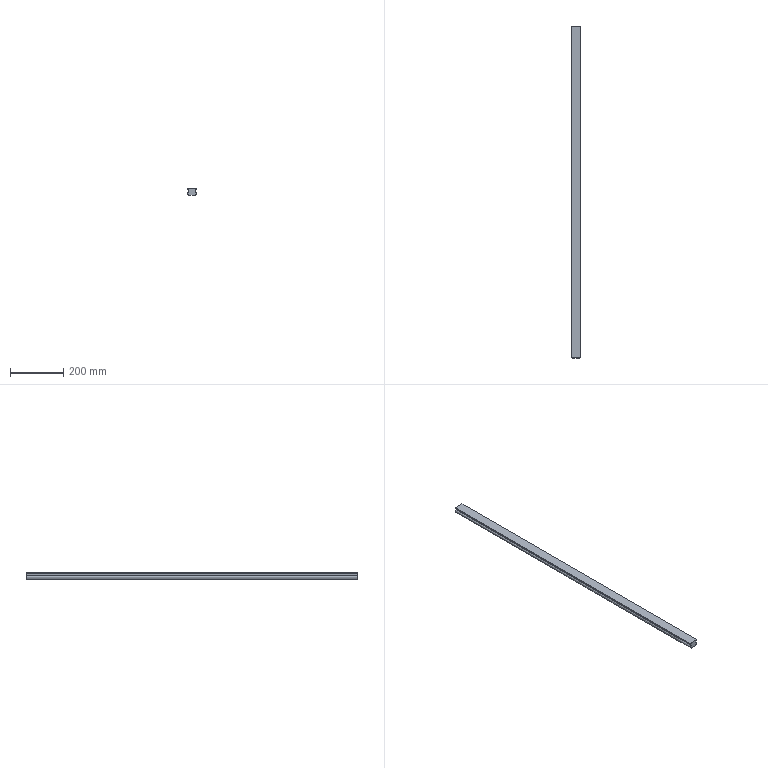Part | SolidWorks | features Extrusion 1 | 1 solid | 14 faces | box 36 x 1252 x 25 mm | volume 935920 mm3 | plane 12 | cylinder 2 | commonest cylinder face diameters 10 x2
STEP:
#1=CARTESIAN_POINT('',(12.5,0.,5.));
#2=VERTEX_POINT('',#1);
#3=CARTESIAN_POINT('',(12.5,0.,-5.));
#4=VERTEX_POINT('',#3);
#5=CARTESIAN_POINT('',(12.5,0.,0.));
#6=DIRECTION('',(0.,1.,0.));
#7=DIRECTION('',(0.,0.,1.));
#8=AXIS2_PLACEMENT_3D('',#5,#6,#7);
#9=CIRCLE('',#8,5.);
#10=EDGE_CURVE('',#2,#4,#9,.T.);
#11=ORIENTED_EDGE('',*,*,#10,.T.);
#12=CARTESIAN_POINT('',(12.5,1252.,-5.));
#13=VERTEX_POINT('',#12);
#14=CARTESIAN_POINT('',(12.5,1252.,-5.));
#15=DIRECTION('',(0.,-1.,0.));
#16=VECTOR('',#15,1000.);
#17=LINE('',#14,#16);
#18=EDGE_CURVE('',#13,#4,#17,.T.);
#19=ORIENTED_EDGE('',*,*,#18,.F.);
#20=CARTESIAN_POINT('',(12.5,1252.,5.));
#21=VERTEX_POINT('',#20);
#22=CARTESIAN_POINT('',(12.5,1252.,0.));
#23=DIRECTION('',(0.,1.,0.));
#24=DIRECTION('',(0.,0.,1.));
#25=AXIS2_PLACEMENT_3D('',#22,#23,#24);
#26=CIRCLE('',#25,5.);
#27=EDGE_CURVE('',#21,#13,#26,.T.);
#28=ORIENTED_EDGE('',*,*,#27,.F.);
#29=CARTESIAN_POINT('',(12.5,1252.,5.));
#30=DIRECTION('',(0.,-1.,0.));
#31=VECTOR('',#30,1000.);
#32=LINE('',#29,#31);
#33=EDGE_CURVE('',#21,#2,#32,.T.);
#34=ORIENTED_EDGE('',*,*,#33,.T.);
#35=EDGE_LOOP('',(#11,#19,#28,#34));
#36=FACE_OUTER_BOUND('',#35,.T.);
#37=CARTESIAN_POINT('',(12.5,1252.,0.));
#38=DIRECTION('',(0.,-1.,0.));
#39=DIRECTION('',(0.,0.,-1.));
#40=AXIS2_PLACEMENT_3D('',#37,#38,#39);
#41=CYLINDRICAL_SURFACE('',#40,5.);
#42=ADVANCED_FACE('',(#36),#41,.T.);
#43=CARTESIAN_POINT('',(12.5,0.,-8.));
#44=VERTEX_POINT('',#43);
#45=CARTESIAN_POINT('',(12.5,0.,-8.));
#46=DIRECTION('',(0.,0.,-1.));
#47=VECTOR('',#46,1000.);
#48=LINE('',#45,#47);
#49=EDGE_CURVE('',#4,#44,#48,.T.);
#50=ORIENTED_EDGE('',*,*,#49,.T.);
#51=CARTESIAN_POINT('',(12.5,1252.,-8.));
#52=VERTEX_POINT('',#51);
#53=CARTESIAN_POINT('',(12.5,1252.,-8.));
#54=DIRECTION('',(0.,-1.,0.));
#55=VECTOR('',#54,1000.);
#56=LINE('',#53,#55);
#57=EDGE_CURVE('',#52,#44,#56,.T.);
#58=ORIENTED_EDGE('',*,*,#57,.F.);
#59=CARTESIAN_POINT('',(12.5,1252.,-8.));
#60=DIRECTION('',(0.,0.,-1.));
#61=VECTOR('',#60,1000.);
#62=LINE('',#59,#61);
#63=EDGE_CURVE('',#13,#52,#62,.T.);
#64=ORIENTED_EDGE('',*,*,#63,.F.);
#65=ORIENTED_EDGE('',*,*,#18,.T.);
#66=EDGE_LOOP('',(#50,#58,#64,#65));
#67=FACE_OUTER_BOUND('',#66,.T.);
#68=CARTESIAN_POINT('',(12.5,1252.,-8.));
#69=DIRECTION('',(-1.,0.,0.));
#70=DIRECTION('',(0.,0.,1.));
#71=AXIS2_PLACEMENT_3D('',#68,#69,#70);
#72=PLANE('',#71);
#73=ADVANCED_FACE('',(#67),#72,.F.);
#74=CARTESIAN_POINT('',(-12.5,0.,-8.));
#75=VERTEX_POINT('',#74);
#76=CARTESIAN_POINT('',(-12.5,0.,-8.));
#77=DIRECTION('',(-1.,0.,0.));
#78=VECTOR('',#77,1000.);
#79=LINE('',#76,#78);
#80=EDGE_CURVE('',#44,#75,#79,.T.);
#81=ORIENTED_EDGE('',*,*,#80,.T.);
#82=CARTESIAN_POINT('',(-12.5,1252.,-8.));
#83=VERTEX_POINT('',#82);
#84=CARTESIAN_POINT('',(-12.5,1252.,-8.));
#85=DIRECTION('',(0.,-1.,0.));
#86=VECTOR('',#85,1000.);
#87=LINE('',#84,#86);
#88=EDGE_CURVE('',#83,#75,#87,.T.);
#89=ORIENTED_EDGE('',*,*,#88,.F.);
#90=CARTESIAN_POINT('',(-12.5,1252.,-8.));
#91=DIRECTION('',(-1.,0.,0.));
#92=VECTOR('',#91,1000.);
#93=LINE('',#90,#92);
#94=EDGE_CURVE('',#52,#83,#93,.T.);
#95=ORIENTED_EDGE('',*,*,#94,.F.);
#96=ORIENTED_EDGE('',*,*,#57,.T.);
#97=EDGE_LOOP('',(#81,#89,#95,#96));
#98=FACE_OUTER_BOUND('',#97,.T.);
#99=CARTESIAN_POINT('',(-12.5,1252.,-8.));
#100=DIRECTION('',(0.,0.,1.));
#101=DIRECTION('',(1.,0.,0.));
#102=AXIS2_PLACEMENT_3D('',#99,#100,#101);
#103=PLANE('',#102);
#104=ADVANCED_FACE('',(#98),#103,.F.);
#105=CARTESIAN_POINT('',(-12.5,0.,-5.));
#106=VERTEX_POINT('',#105);
#107=CARTESIAN_POINT('',(-12.5,0.,-5.));
#108=DIRECTION('',(0.,0.,1.));
#109=VECTOR('',#108,1000.);
#110=LINE('',#107,#109);
#111=EDGE_CURVE('',#75,#106,#110,.T.);
#112=ORIENTED_EDGE('',*,*,#111,.T.);
#113=CARTESIAN_POINT('',(-12.5,1252.,-5.));
#114=VERTEX_POINT('',#113);
#115=CARTESIAN_POINT('',(-12.5,1252.,-5.));
#116=DIRECTION('',(0.,-1.,0.));
#117=VECTOR('',#116,1000.);
#118=LINE('',#115,#117);
#119=EDGE_CURVE('',#114,#106,#118,.T.);
#120=ORIENTED_EDGE('',*,*,#119,.F.);
#121=CARTESIAN_POINT('',(-12.5,1252.,-5.));
#122=DIRECTION('',(0.,0.,1.));
#123=VECTOR('',#122,1000.);
#124=LINE('',#121,#123);
#125=EDGE_CURVE('',#83,#114,#124,.T.);
#126=ORIENTED_EDGE('',*,*,#125,.F.);
#127=ORIENTED_EDGE('',*,*,#88,.T.);
#128=EDGE_LOOP('',(#112,#120,#126,#127));
#129=FACE_OUTER_BOUND('',#128,.T.);
#130=CARTESIAN_POINT('',(-12.5,1252.,-5.));
#131=DIRECTION('',(1.,0.,0.));
#132=DIRECTION('',(0.,0.,-1.));
#133=AXIS2_PLACEMENT_3D('',#130,#131,#132);
#134=PLANE('',#133);
#135=ADVANCED_FACE('',(#129),#134,.F.);
#136=CARTESIAN_POINT('',(-12.5,0.,5.));
#137=VERTEX_POINT('',#136);
#138=CARTESIAN_POINT('',(-12.5,0.,0.));
#139=DIRECTION('',(0.,1.,0.));
#140=DIRECTION('',(0.,0.,1.));
#141=AXIS2_PLACEMENT_3D('',#138,#139,#140);
#142=CIRCLE('',#141,5.);
#143=EDGE_CURVE('',#106,#137,#142,.T.);
#144=ORIENTED_EDGE('',*,*,#143,.T.);
#145=CARTESIAN_POINT('',(-12.5,1252.,5.));
#146=VERTEX_POINT('',#145);
#147=CARTESIAN_POINT('',(-12.5,1252.,5.));
#148=DIRECTION('',(0.,-1.,0.));
#149=VECTOR('',#148,1000.);
#150=LINE('',#147,#149);
#151=EDGE_CURVE('',#146,#137,#150,.T.);
#152=ORIENTED_EDGE('',*,*,#151,.F.);
#153=CARTESIAN_POINT('',(-12.5,1252.,0.));
#154=DIRECTION('',(0.,1.,0.));
#155=DIRECTION('',(0.,0.,1.));
#156=AXIS2_PLACEMENT_3D('',#153,#154,#155);
#157=CIRCLE('',#156,5.);
#158=EDGE_CURVE('',#114,#146,#157,.T.);
#159=ORIENTED_EDGE('',*,*,#158,.F.);
#160=ORIENTED_EDGE('',*,*,#119,.T.);
#161=EDGE_LOOP('',(#144,#152,#159,#160));
#162=FACE_OUTER_BOUND('',#161,.T.);
#163=CARTESIAN_POINT('',(-12.5,1252.,0.));
#164=DIRECTION('',(0.,-1.,0.));
#165=DIRECTION('',(0.,0.,-1.));
#166=AXIS2_PLACEMENT_3D('',#163,#164,#165);
#167=CYLINDRICAL_SURFACE('',#166,5.);
#168=ADVANCED_FACE('',(#162),#167,.T.);
#169=CARTESIAN_POINT('',(-12.5,0.,13.));
#170=VERTEX_POINT('',#169);
#171=CARTESIAN_POINT('',(-12.5,0.,5.));
#172=DIRECTION('',(0.,0.,1.));
#173=VECTOR('',#172,1000.);
#174=LINE('',#171,#173);
#175=EDGE_CURVE('',#137,#170,#174,.T.);
#176=ORIENTED_EDGE('',*,*,#175,.T.);
#177=CARTESIAN_POINT('',(-12.5,1252.,13.));
#178=VERTEX_POINT('',#177);
#179=CARTESIAN_POINT('',(-12.5,1252.,13.));
#180=DIRECTION('',(0.,-1.,0.));
#181=VECTOR('',#180,1000.);
#182=LINE('',#179,#181);
#183=EDGE_CURVE('',#178,#170,#182,.T.);
#184=ORIENTED_EDGE('',*,*,#183,.F.);
#185=CARTESIAN_POINT('',(-12.5,1252.,5.));
#186=DIRECTION('',(0.,0.,1.));
#187=VECTOR('',#186,1000.);
#188=LINE('',#185,#187);
#189=EDGE_CURVE('',#146,#178,#188,.T.);
#190=ORIENTED_EDGE('',*,*,#189,.F.);
#191=ORIENTED_EDGE('',*,*,#151,.T.);
#192=EDGE_LOOP('',(#176,#184,#190,#191));
#193=FACE_OUTER_BOUND('',#192,.T.);
#194=CARTESIAN_POINT('',(-12.5,1252.,5.));
#195=DIRECTION('',(1.,0.,0.));
#196=DIRECTION('',(0.,0.,-1.));
#197=AXIS2_PLACEMENT_3D('',#194,#195,#196);
#198=PLANE('',#197);
#199=ADVANCED_FACE('',(#193),#198,.F.);
#200=CARTESIAN_POINT('',(-18.,0.,13.));
#201=VERTEX_POINT('',#200);
#202=CARTESIAN_POINT('',(-12.5,0.,13.));
#203=DIRECTION('',(-1.,0.,0.));
#204=VECTOR('',#203,1000.);
#205=LINE('',#202,#204);
#206=EDGE_CURVE('',#170,#201,#205,.T.);
#207=ORIENTED_EDGE('',*,*,#206,.T.);
#208=CARTESIAN_POINT('',(-18.,1252.,13.));
#209=VERTEX_POINT('',#208);
#210=CARTESIAN_POINT('',(-18.,1252.,13.));
#211=DIRECTION('',(0.,-1.,0.));
#212=VECTOR('',#211,1000.);
#213=LINE('',#210,#212);
#214=EDGE_CURVE('',#209,#201,#213,.T.);
#215=ORIENTED_EDGE('',*,*,#214,.F.);
#216=CARTESIAN_POINT('',(-12.5,1252.,13.));
#217=DIRECTION('',(-1.,0.,0.));
#218=VECTOR('',#217,1000.);
#219=LINE('',#216,#218);
#220=EDGE_CURVE('',#178,#209,#219,.T.);
#221=ORIENTED_EDGE('',*,*,#220,.F.);
#222=ORIENTED_EDGE('',*,*,#183,.T.);
#223=EDGE_LOOP('',(#207,#215,#221,#222));
#224=FACE_OUTER_BOUND('',#223,.T.);
#225=CARTESIAN_POINT('',(-12.5,1252.,13.));
#226=DIRECTION('',(0.,0.,1.));
#227=DIRECTION('',(1.,0.,0.));
#228=AXIS2_PLACEMENT_3D('',#225,#226,#227);
#229=PLANE('',#228);
#230=ADVANCED_FACE('',(#224),#229,.F.);
#231=CARTESIAN_POINT('',(-18.,0.,17.));
#232=VERTEX_POINT('',#231);
#233=CARTESIAN_POINT('',(-18.,0.,13.));
#234=DIRECTION('',(0.,0.,1.));
#235=VECTOR('',#234,1000.);
#236=LINE('',#233,#235);
#237=EDGE_CURVE('',#201,#232,#236,.T.);
#238=ORIENTED_EDGE('',*,*,#237,.T.);
#239=CARTESIAN_POINT('',(-18.,1252.,17.));
#240=VERTEX_POINT('',#239);
#241=CARTESIAN_POINT('',(-18.,1252.,17.));
#242=DIRECTION('',(0.,-1.,0.));
#243=VECTOR('',#242,1000.);
#244=LINE('',#241,#243);
#245=EDGE_CURVE('',#240,#232,#244,.T.);
#246=ORIENTED_EDGE('',*,*,#245,.F.);
#247=CARTESIAN_POINT('',(-18.,1252.,13.));
#248=DIRECTION('',(0.,0.,1.));
#249=VECTOR('',#248,1000.);
#250=LINE('',#247,#249);
#251=EDGE_CURVE('',#209,#240,#250,.T.);
#252=ORIENTED_EDGE('',*,*,#251,.F.);
#253=ORIENTED_EDGE('',*,*,#214,.T.);
#254=EDGE_LOOP('',(#238,#246,#252,#253));
#255=FACE_OUTER_BOUND('',#254,.T.);
#256=CARTESIAN_POINT('',(-18.,1252.,13.));
#257=DIRECTION('',(1.,0.,0.));
#258=DIRECTION('',(0.,0.,-1.));
#259=AXIS2_PLACEMENT_3D('',#256,#257,#258);
#260=PLANE('',#259);
#261=ADVANCED_FACE('',(#255),#260,.F.);
#262=CARTESIAN_POINT('',(18.,0.,17.));
#263=VERTEX_POINT('',#262);
#264=CARTESIAN_POINT('',(-18.,0.,17.));
#265=DIRECTION('',(1.,0.,0.));
#266=VECTOR('',#265,1000.);
#267=LINE('',#264,#266);
#268=EDGE_CURVE('',#232,#263,#267,.T.);
#269=ORIENTED_EDGE('',*,*,#268,.T.);
#270=CARTESIAN_POINT('',(18.,1252.,17.));
#271=VERTEX_POINT('',#270);
#272=CARTESIAN_POINT('',(18.,1252.,17.));
#273=DIRECTION('',(0.,-1.,0.));
#274=VECTOR('',#273,1000.);
#275=LINE('',#272,#274);
#276=EDGE_CURVE('',#271,#263,#275,.T.);
#277=ORIENTED_EDGE('',*,*,#276,.F.);
#278=CARTESIAN_POINT('',(-18.,1252.,17.));
#279=DIRECTION('',(1.,0.,0.));
#280=VECTOR('',#279,1000.);
#281=LINE('',#278,#280);
#282=EDGE_CURVE('',#240,#271,#281,.T.);
#283=ORIENTED_EDGE('',*,*,#282,.F.);
#284=ORIENTED_EDGE('',*,*,#245,.T.);
#285=EDGE_LOOP('',(#269,#277,#283,#284));
#286=FACE_OUTER_BOUND('',#285,.T.);
#287=CARTESIAN_POINT('',(-18.,1252.,17.));
#288=DIRECTION('',(0.,0.,-1.));
#289=DIRECTION('',(-1.,0.,0.));
#290=AXIS2_PLACEMENT_3D('',#287,#288,#289);
#291=PLANE('',#290);
#292=ADVANCED_FACE('',(#286),#291,.F.);
#293=CARTESIAN_POINT('',(18.,0.,13.));
#294=VERTEX_POINT('',#293);
#295=CARTESIAN_POINT('',(18.,0.,17.));
#296=DIRECTION('',(0.,0.,-1.));
#297=VECTOR('',#296,1000.);
#298=LINE('',#295,#297);
#299=EDGE_CURVE('',#263,#294,#298,.T.);
#300=ORIENTED_EDGE('',*,*,#299,.T.);
#301=CARTESIAN_POINT('',(18.,1252.,13.));
#302=VERTEX_POINT('',#301);
#303=CARTESIAN_POINT('',(18.,1252.,13.));
#304=DIRECTION('',(0.,-1.,0.));
#305=VECTOR('',#304,1000.);
#306=LINE('',#303,#305);
#307=EDGE_CURVE('',#302,#294,#306,.T.);
#308=ORIENTED_EDGE('',*,*,#307,.F.);
#309=CARTESIAN_POINT('',(18.,1252.,17.));
#310=DIRECTION('',(0.,0.,-1.));
#311=VECTOR('',#310,1000.);
#312=LINE('',#309,#311);
#313=EDGE_CURVE('',#271,#302,#312,.T.);
#314=ORIENTED_EDGE('',*,*,#313,.F.);
#315=ORIENTED_EDGE('',*,*,#276,.T.);
#316=EDGE_LOOP('',(#300,#308,#314,#315));
#317=FACE_OUTER_BOUND('',#316,.T.);
#318=CARTESIAN_POINT('',(18.,1252.,17.));
#319=DIRECTION('',(-1.,0.,0.));
#320=DIRECTION('',(0.,0.,1.));
#321=AXIS2_PLACEMENT_3D('',#318,#319,#320);
#322=PLANE('',#321);
#323=ADVANCED_FACE('',(#317),#322,.F.);
#324=CARTESIAN_POINT('',(12.5,0.,13.));
#325=VERTEX_POINT('',#324);
#326=CARTESIAN_POINT('',(18.,0.,13.));
#327=DIRECTION('',(-1.,0.,0.));
#328=VECTOR('',#327,1000.);
#329=LINE('',#326,#328);
#330=EDGE_CURVE('',#294,#325,#329,.T.);
#331=ORIENTED_EDGE('',*,*,#330,.T.);
#332=CARTESIAN_POINT('',(12.5,1252.,13.));
#333=VERTEX_POINT('',#332);
#334=CARTESIAN_POINT('',(12.5,1252.,13.));
#335=DIRECTION('',(0.,-1.,0.));
#336=VECTOR('',#335,1000.);
#337=LINE('',#334,#336);
#338=EDGE_CURVE('',#333,#325,#337,.T.);
#339=ORIENTED_EDGE('',*,*,#338,.F.);
#340=CARTESIAN_POINT('',(18.,1252.,13.));
#341=DIRECTION('',(-1.,0.,0.));
#342=VECTOR('',#341,1000.);
#343=LINE('',#340,#342);
#344=EDGE_CURVE('',#302,#333,#343,.T.);
#345=ORIENTED_EDGE('',*,*,#344,.F.);
#346=ORIENTED_EDGE('',*,*,#307,.T.);
#347=EDGE_LOOP('',(#331,#339,#345,#346));
#348=FACE_OUTER_BOUND('',#347,.T.);
#349=CARTESIAN_POINT('',(18.,1252.,13.));
#350=DIRECTION('',(0.,0.,1.));
#351=DIRECTION('',(1.,0.,0.));
#352=AXIS2_PLACEMENT_3D('',#349,#350,#351);
#353=PLANE('',#352);
#354=ADVANCED_FACE('',(#348),#353,.F.);
#355=CARTESIAN_POINT('',(12.5,0.,13.));
#356=DIRECTION('',(0.,0.,-1.));
#357=VECTOR('',#356,1000.);
#358=LINE('',#355,#357);
#359=EDGE_CURVE('',#325,#2,#358,.T.);
#360=ORIENTED_EDGE('',*,*,#359,.T.);
#361=ORIENTED_EDGE('',*,*,#33,.F.);
#362=CARTESIAN_POINT('',(12.5,1252.,13.));
#363=DIRECTION('',(0.,0.,-1.));
#364=VECTOR('',#363,1000.);
#365=LINE('',#362,#364);
#366=EDGE_CURVE('',#333,#21,#365,.T.);
#367=ORIENTED_EDGE('',*,*,#366,.F.);
#368=ORIENTED_EDGE('',*,*,#338,.T.);
#369=EDGE_LOOP('',(#360,#361,#367,#368));
#370=FACE_OUTER_BOUND('',#369,.T.);
#371=CARTESIAN_POINT('',(12.5,1252.,13.));
#372=DIRECTION('',(-1.,0.,0.));
#373=DIRECTION('',(0.,0.,1.));
#374=AXIS2_PLACEMENT_3D('',#371,#372,#373);
#375=PLANE('',#374);
#376=ADVANCED_FACE('',(#370),#375,.F.);
#377=ORIENTED_EDGE('',*,*,#27,.T.);
#378=ORIENTED_EDGE('',*,*,#63,.T.);
#379=ORIENTED_EDGE('',*,*,#94,.T.);
#380=ORIENTED_EDGE('',*,*,#125,.T.);
#381=ORIENTED_EDGE('',*,*,#158,.T.);
#382=ORIENTED_EDGE('',*,*,#189,.T.);
#383=ORIENTED_EDGE('',*,*,#220,.T.);
#384=ORIENTED_EDGE('',*,*,#251,.T.);
#385=ORIENTED_EDGE('',*,*,#282,.T.);
#386=ORIENTED_EDGE('',*,*,#313,.T.);
#387=ORIENTED_EDGE('',*,*,#344,.T.);
#388=ORIENTED_EDGE('',*,*,#366,.T.);
#389=EDGE_LOOP('',(#377,#378,#379,#380,#381,#382,#383,#384,#385,#386,#387,#388));
#390=FACE_OUTER_BOUND('',#389,.T.);
#391=CARTESIAN_POINT('',(12.5,1252.,0.));
#392=DIRECTION('',(0.,1.,0.));
#393=DIRECTION('',(0.,0.,1.));
#394=AXIS2_PLACEMENT_3D('',#391,#392,#393);
#395=PLANE('',#394);
#396=ADVANCED_FACE('',(#390),#395,.T.);
#397=ORIENTED_EDGE('',*,*,#10,.F.);
#398=ORIENTED_EDGE('',*,*,#359,.F.);
#399=ORIENTED_EDGE('',*,*,#330,.F.);
#400=ORIENTED_EDGE('',*,*,#299,.F.);
#401=ORIENTED_EDGE('',*,*,#268,.F.);
#402=ORIENTED_EDGE('',*,*,#237,.F.);
#403=ORIENTED_EDGE('',*,*,#206,.F.);
#404=ORIENTED_EDGE('',*,*,#175,.F.);
#405=ORIENTED_EDGE('',*,*,#143,.F.);
#406=ORIENTED_EDGE('',*,*,#111,.F.);
#407=ORIENTED_EDGE('',*,*,#80,.F.);
#408=ORIENTED_EDGE('',*,*,#49,.F.);
#409=EDGE_LOOP('',(#397,#398,#399,#400,#401,#402,#403,#404,#405,#406,#407,#408));
#410=FACE_OUTER_BOUND('',#409,.T.);
#411=CARTESIAN_POINT('',(12.5,0.,0.));
#412=DIRECTION('',(0.,1.,0.));
#413=DIRECTION('',(0.,0.,1.));
#414=AXIS2_PLACEMENT_3D('',#411,#412,#413);
#415=PLANE('',#414);
#416=ADVANCED_FACE('',(#410),#415,.F.);
#417=CLOSED_SHELL('',(#42,#73,#104,#135,#168,#199,#230,#261,#292,#323,#354,#376,#396,#416));
#418=MANIFOLD_SOLID_BREP('',#417);
#419=CARTESIAN_POINT('',(0.,0.,0.));
#420=DIRECTION('',(0.,0.,1.));
#421=DIRECTION('',(1.,0.,0.));
#422=AXIS2_PLACEMENT_3D('',#419,#420,#421);
#423=(LENGTH_UNIT()NAMED_UNIT(*)SI_UNIT(.MILLI.,.METRE.));
#424=UNCERTAINTY_MEASURE_WITH_UNIT(LENGTH_MEASURE(0.00001),#423,'','');
#425=(NAMED_UNIT(*)PLANE_ANGLE_UNIT()SI_UNIT($,.RADIAN.));
#426=(NAMED_UNIT(*)SI_UNIT($,.STERADIAN.)SOLID_ANGLE_UNIT());
#427=(GEOMETRIC_REPRESENTATION_CONTEXT(3)GLOBAL_UNCERTAINTY_ASSIGNED_CONTEXT((#424))GLOBAL_UNIT_ASSIGNED_CONTEXT((#423,#425,#426))REPRESENTATION_CONTEXT('',''));
#428=ADVANCED_BREP_SHAPE_REPRESENTATION('',(#418,#422),#427);